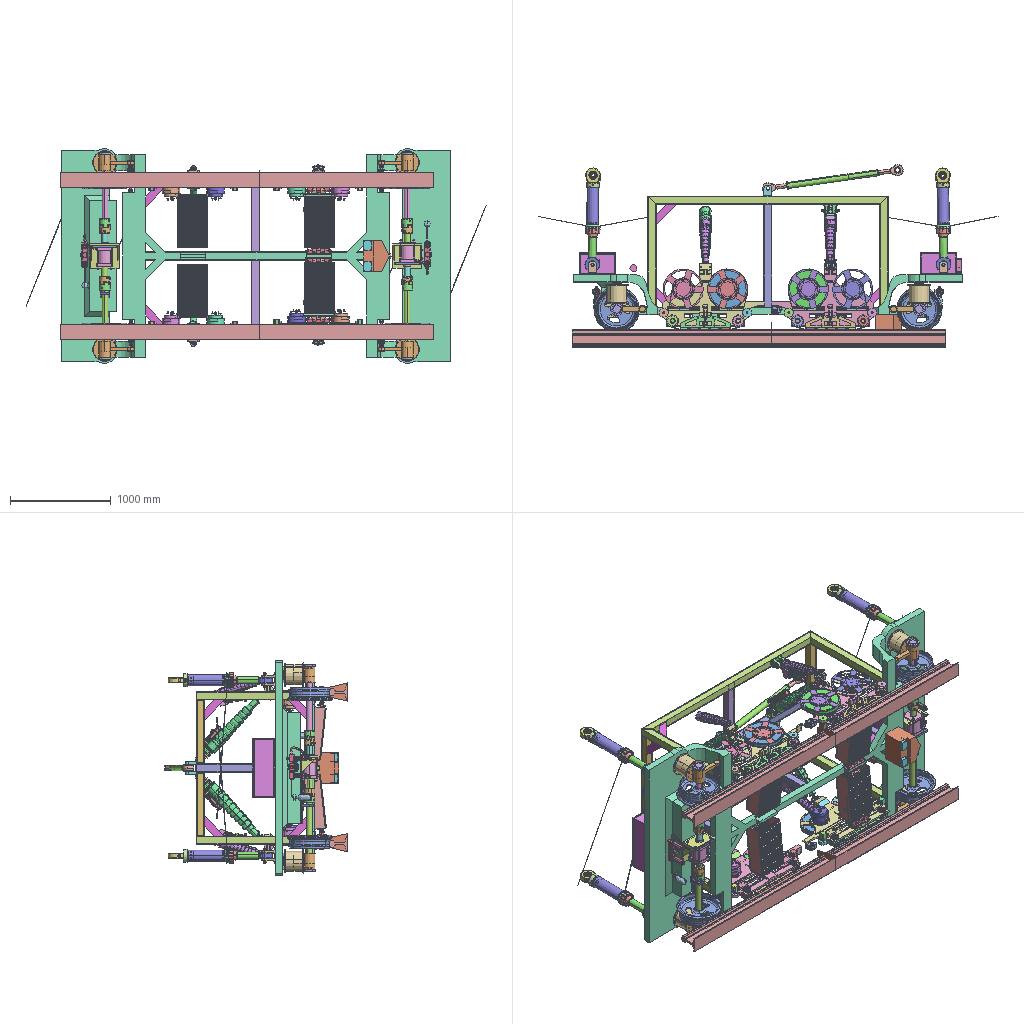Assembly | STEP file | 122 different items | 810 placed | box 4562 x 1815 x 2130 mm
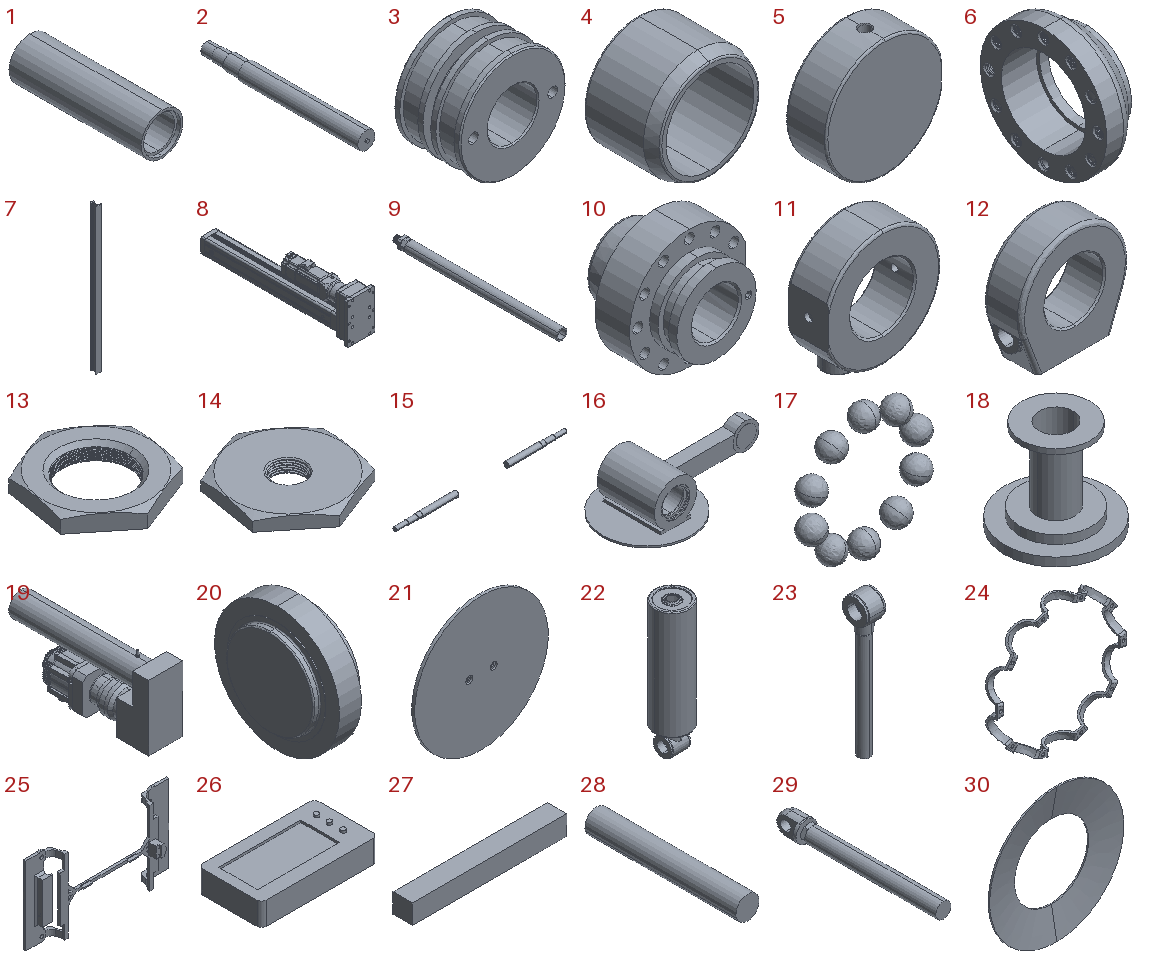Parts list (item | name | quantity | parent item | size | volume):
1 | 1. Barrel | x4 | in Hydraulic cylinder | 114.3 x 362.5 x 114.3 mm | 1450450 mm3
2 | 2. Piston Rod | x4 | in Hydraulic cylinder | 71.582 x 670.101 x 71.582 mm | 2394238 mm3
3 | 3. Piston | x4 | in Hydraulic cylinder | 88.35 x 55 x 88.35 mm | 216858 mm3
4 | 4. Piston Cap | x4 | in Hydraulic cylinder | 60 x 40 x 60 mm | 35974 mm3
5 | 5. End Cap | x4 | in Hydraulic cylinder | - | -
6 | 6. Barrel Cap | x4 | in Hydraulic cylinder | - | -
7 | 60 rail | x2 | - | 150 x 176.167 x 3700 mm | 28206021 mm3
8 | 60-400mm cylinder body | x2 | in 60-400mm branch 12 | - | -
9 | 60-400mm push rod | x2 | in 60-400mm branch 12 | 35 x 555 x 35 mm | 228632 mm3
10 | 7. Front Cap | x4 | in Hydraulic cylinder | - | -
11 | 8. Front Clevis | x4 | in Hydraulic cylinder | - | -
12 | 9. Rear Clevis | x4 | in Hydraulic cylinder | 146 x 50.8 x 148 mm | 646716 mm3
13 | Adjusting nut 1 | x4 | in Axle box spring | 86.085 x 91.305 x 12 mm | 42133 mm3
14 | Adjusting nut 2 | x4 | in VSVDMRD | 53.803 x 57.066 x 6 mm | 11857 mm3
15 | Axle | x2 | - | 2025 x 64 x 64 mm | 3440421 mm3
16 | Axle box 1 | x4 | - | 410 x 240 x 120.8 mm | 1300329 mm3
17 | Ball | x16 | in Ball Bearing | 70.063 x 13 x 73 mm | 11503 mm3
18 | Base | x4 | in VSVDMRD | 60 x 60 x 53 mm | 24076 mm3
19 | Base body | x2 | in Multi-stage cylinder assembly | 90 x 360 x 196.75 mm | 2809262 mm3
20 | Bearing end cap 1 | x4 | - | 39.936 x 120.436 x 120.436 mm | 192561 mm3
21 | Bottom cover | x4 | in Housing assembly | 230 x 5 x 230 mm | 206946 mm3
22 | C40-55H | x4 | in 22 | - | -
23 | C40-55H-1 | x4 | in 22 | - | -
24 | Case | x32 | in Ball Bearing | 63.56 x 7.5 x 63.56 mm | 756.109 mm3
25 | Chassis | x1 | - | 3860 x 630 x 2130 mm | 286011654 mm3
26 | Controller | x1 | - | 254.791 x 138.794 x 55 mm | 1688527 mm3
27 | Crossbeam | x3 | - | 635 x 80 x 80 mm | 1850000 mm3
28 | Cylinder 1 | x2 | in Multi-stage cylinder assembly | 46 x 300 x 46 mm | 498571 mm3
29 | Cylinder 2 | x2 | in Multi-stage cylinder assembly | 48 x 372 x 48.4 mm | 366109 mm3
30 | Disc spring | x48 | in Disc spring stack | 90 x 4.485 x 90 mm | 4464 mm3
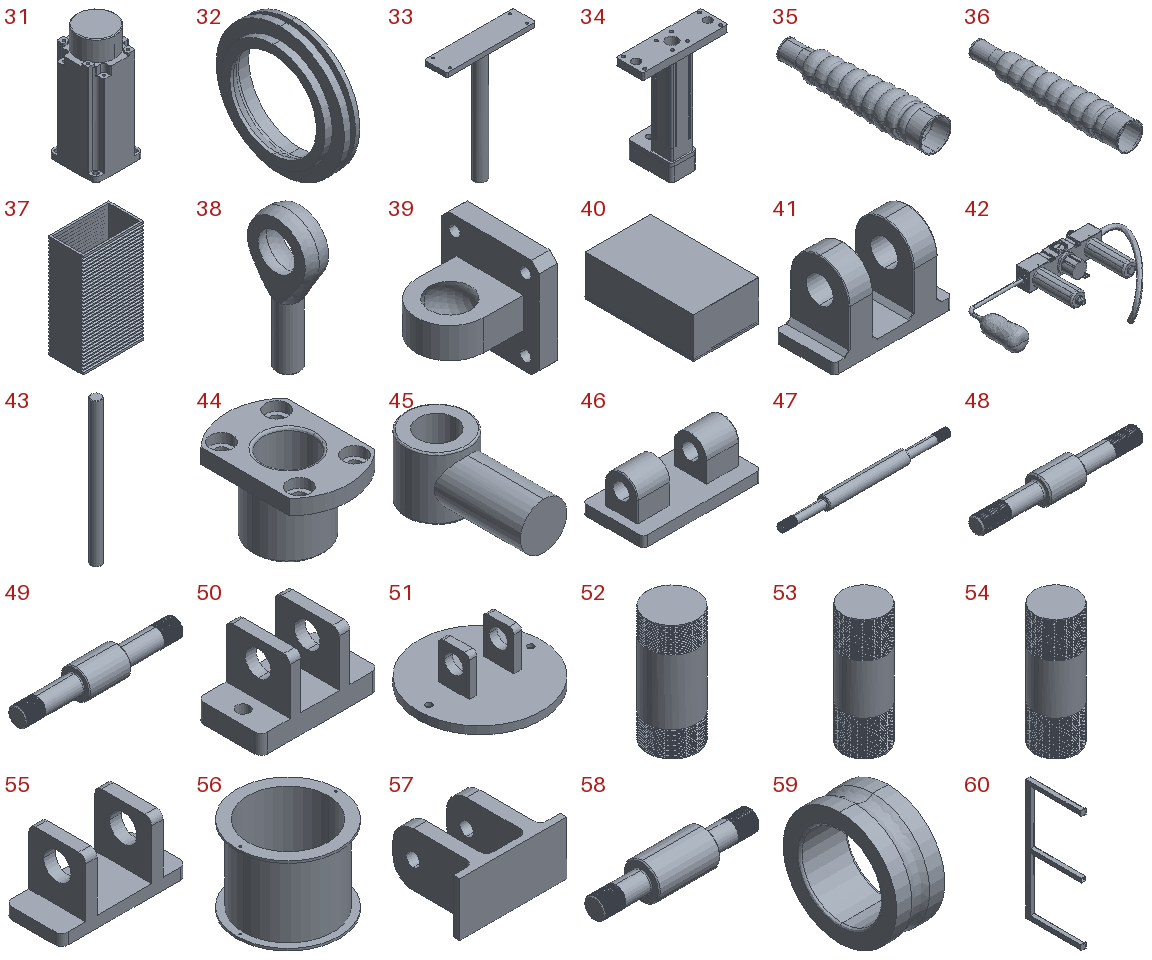31 | Drive motor | x2 | in Electric cylinder with guide post | 60 x 60 x 146.5 mm | 432413 mm3
32 | Dust ring 1 | x2 | - | 15.692 x 75.322 x 75.322 mm | 18737 mm3
33 | Electric cylinder assembly 1 | x2 | in Electric cylinder with guide post | 295 x 75 x 394 mm | 805333 mm3
34 | Electric cylinder assembly 2 | x2 | in Electric cylinder with guide post | 295 x 157.01 x 389 mm | 2717250 mm3
35 | Electric cylinder dust boot, cylinder A | x4 | - | 98.284 x 439.582 x 98.284 mm | 200790 mm3
36 | Electric cylinder dust boot, cylinder B | x4 | - | 122.855 x 671.584 x 122.855 mm | 479397 mm3
37 | Electric cylinder dust boot, cylinder C | x4 | - | 300 x 172 x 510 mm | 3753035 mm3
38 | Electric cylinder end | x2 | in 60-400mm branch 12 | 20 x 53.333 x 116.667 mm | 46086 mm3
39 | Electric cylinder rear end | x2 | in 60-400mm branch 12 | 102.201 x 110.238 x 110 mm | 342239 mm3
40 | Electrical box | x2 | - | - | 11408010 mm3
41 | Frame R-pair hinge lug | x4 | in 打磨单元与电动缸-3支链-铰接点加宽, 打磨单元与电动缸Mirror-3支链-铰接点加宽 | 140 x 70 x 98 mm | 392765 mm3
42 | GC300-400 FRL air unit [GC400-15]_GC400-15 | x2 | in CS2 series standard pneumatic cylinder [CDS2F140-100]_CDS2F140-100 | 534.272 x 247.073 x 161.659 mm | 1621507 mm3
43 | Guide post | x4 | in Electric cylinder with guide post | 20 x 20 x 280 mm | 87904 mm3
44 | Guide post flange | x4 | in Electric cylinder with guide post | 34 x 49 x 30 mm | 13227 mm3
45 | Hinge | x4 | in VSVDMRD | 20 x 44.5 x 20 mm | 8479 mm3
46 | Hinge lug widened | x4 | in Electric cylinder with guide post | 145 x 75 x 58 mm | 246181 mm3
47 | Hinge pin stepped shaft | x4 | in Hinge assembly M20 spacing 20 | 260 x 20 x 20 mm | 54217 mm3
48 | Hinge pin stepped shaft 1 | x4 | in Unit hinge short shaft | 120 x 20 x 20 mm | 18916 mm3
49 | Hinge pin stepped shaft 2 | x4 | in Frame hinge short shaft | 172 x 32 x 32 mm | 76081 mm3
50 | Hinge seat | x4 | in Axle box spring | 55 x 30 x 34 mm | 20602 mm3
51 | Hinge seat 1 | x4 | in Axle box spring | 80 x 80 x 30 mm | 28682 mm3
52 | Hinge seat cylinder | x4 | in Axle box spring | 12 x 12 x 28 mm | 3114 mm3
53 | Hinge seat cylinder 1 | x4 | in Axle box spring | 12 x 12 x 34 mm | 3769 mm3
54 | Hinge seat cylinder 3 | x8 | in VSVDMRD | 12 x 12 x 34 mm | 3769 mm3
55 | Hinge top seat 3 | x8 | in VSVDMRD | 55 x 25 x 30 mm | 11917 mm3
56 | Housing | x4 | in Housing assembly | 230 x 230 x 175 mm | 1145645 mm3
57 | Hydraulic cylinder base | x4 | - | 160 x 130 x 80 mm | 490850 mm3
58 | Hydraulic cylinder hinge pin stepped shaft | x4 | - | 152 x 35 x 35 mm | 86130 mm3
59 | Inner Ring | x16 | in Ball Bearing | 21 x 49.56 x 49.56 mm | 19228 mm3
60 | Inner frame 1 | x1 | - | 100 x 1100 x 2400 mm | 8328429 mm3
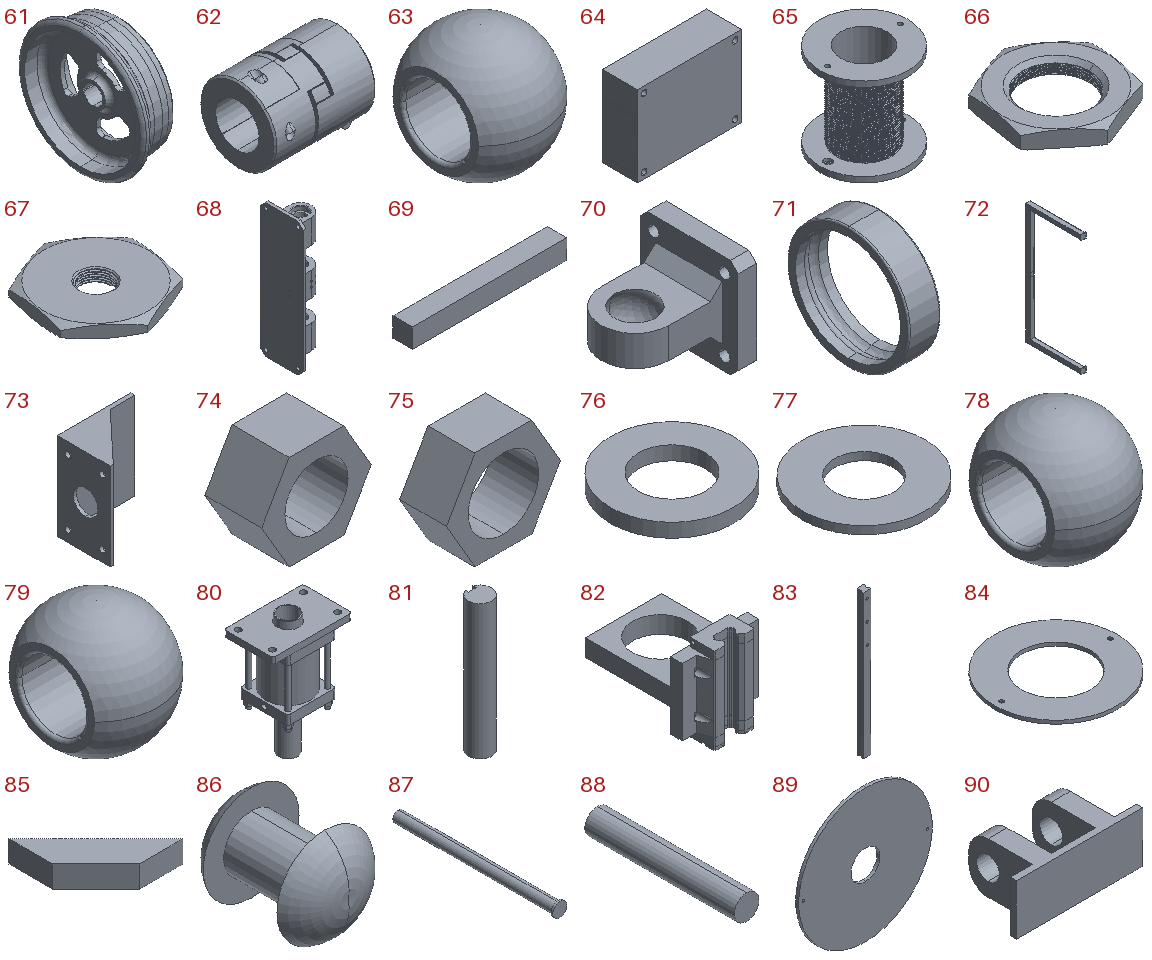61 | LM wheel | x4 | - | 135 x 449.742 x 449.742 mm | 4161570 mm3
62 | LYCA jaw coupling [LYCA-105140]_LYCA-105140 | x4 | in CS2 series standard pneumatic cylinder [CDS2F140-100]_CDS2F140-100 | 140 x 108.875 x 107.681 mm | 781609 mm3
63 | Large rod end bearing | x2 | in 60-400mm branch 12 | 42.667 x 59.28 x 59.28 mm | 62997 mm3
64 | Laser ranging sensor 1200mm | x2 | - | 92 x 31 x 71 mm | 199839 mm3
65 | Load-bearing column 1 | x4 | in Axle box spring | 80 x 80 x 80 mm | 74344 mm3
66 | Lock nut | x4 | in Axle box spring | 86.085 x 91.305 x 12 mm | 41343 mm3
67 | Lock nut 2 | x4 | in VSVDMRD | 53.803 x 57.066 x 6 mm | 11722 mm3
68 | Lower hinge plate thickness 20 widened | x4 | in 打磨单元与电动缸-3支链-铰接点加宽, 打磨单元与电动缸Mirror-3支链-铰接点加宽 | 55 x 80 x 248 mm | 298124 mm3
69 | Middle crossbeam | x2 | - | 635 x 80 x 80 mm | 1850000 mm3
70 | Multi-stage electric cylinder rear end | x2 | in Multi-stage cylinder assembly | 90.745 x 85.184 x 85 mm | 182065 mm3
71 | Outer Ring | x16 | in Ball Bearing | 21 x 80 x 80 mm | 23803 mm3
72 | Outer frame 1 | x2 | - | 100 x 1100 x 2400 mm | 6796800 mm3
73 | Part 2 | x2 | - | 240 x 172.72 x 285 mm | 1617851 mm3
74 | Pin shaft nut M12 | x16 | in Hinge assembly M20 spacing 20, Unit hinge short shaft | 20.785 x 10.8 x 18 mm | 1809 mm3
75 | Pin shaft nut M20 | x8 | in Frame hinge short shaft | 32.332 x 13.3 x 28 mm | 4852 mm3
76 | Pin washer nut at M12 | x8 | in Unit hinge short shaft | 24 x 24 x 2.7 mm | 863.074 mm3
77 | Pin washer nut at M20 | x8 | in Frame hinge short shaft | 42 x 42 x 2.7 mm | 2892 mm3
78 | Rod end bearing | x2 | in 60-400mm branch 12 | 26.667 x 37.05 x 37.05 mm | 15380 mm3
79 | Rod end bearing 1 | x2 | in Traction tie rod | 56 x 77.805 x 77.805 mm | 142436 mm3
80 | - | x2 | in CS2 series standard pneumatic cylinder [CDS2F140-100]_CDS2F140-100 | 255 x 160 x 391 mm | 4492396 mm3
81 | - | x2 | in CS2 series standard pneumatic cylinder [CDS2F140-100]_CDS2F140-100 | 60 x 60 x 350 mm | 980167 mm3
82 | - | x2 | in HGW-CC, HGW-HC ball linear guide [HGW25HCE1R160EZ0CI+E2╱RC] | 90 x 130.4 x 101.35 mm | 273485 mm3
83 | - | x2 | in HGW-CC, HGW-HC ball linear guide [HGW25HCE1R160EZ0CI+E2╱RC] | 23 x 22 x 429 mm | 189571 mm3
84 | Spacer block | x4 | in Axle box spring | 180 x 180 x 5 mm | 87215 mm3
85 | Support rib 1 | x10 | - | 200 x 200 x 50 mm | 750000 mm3
86 | Szegecs | x160 | in Ball Bearing | 2.6 x 3.322 x 2.6 mm | 7.735 mm3
87 | Tie rod | x1 | in Traction tie rod | 80 x 910 x 80 mm | 827810 mm3
88 | Tie rod 2 | x1 | in Traction tie rod | 50 x 300 x 50 mm | 589049 mm3
89 | Top cover | x4 | in Housing assembly | 230 x 5 x 230 mm | 197795 mm3
90 | Traction rod base | x1 | in Traction tie rod | 200 x 110 x 80 mm | 555750 mm3
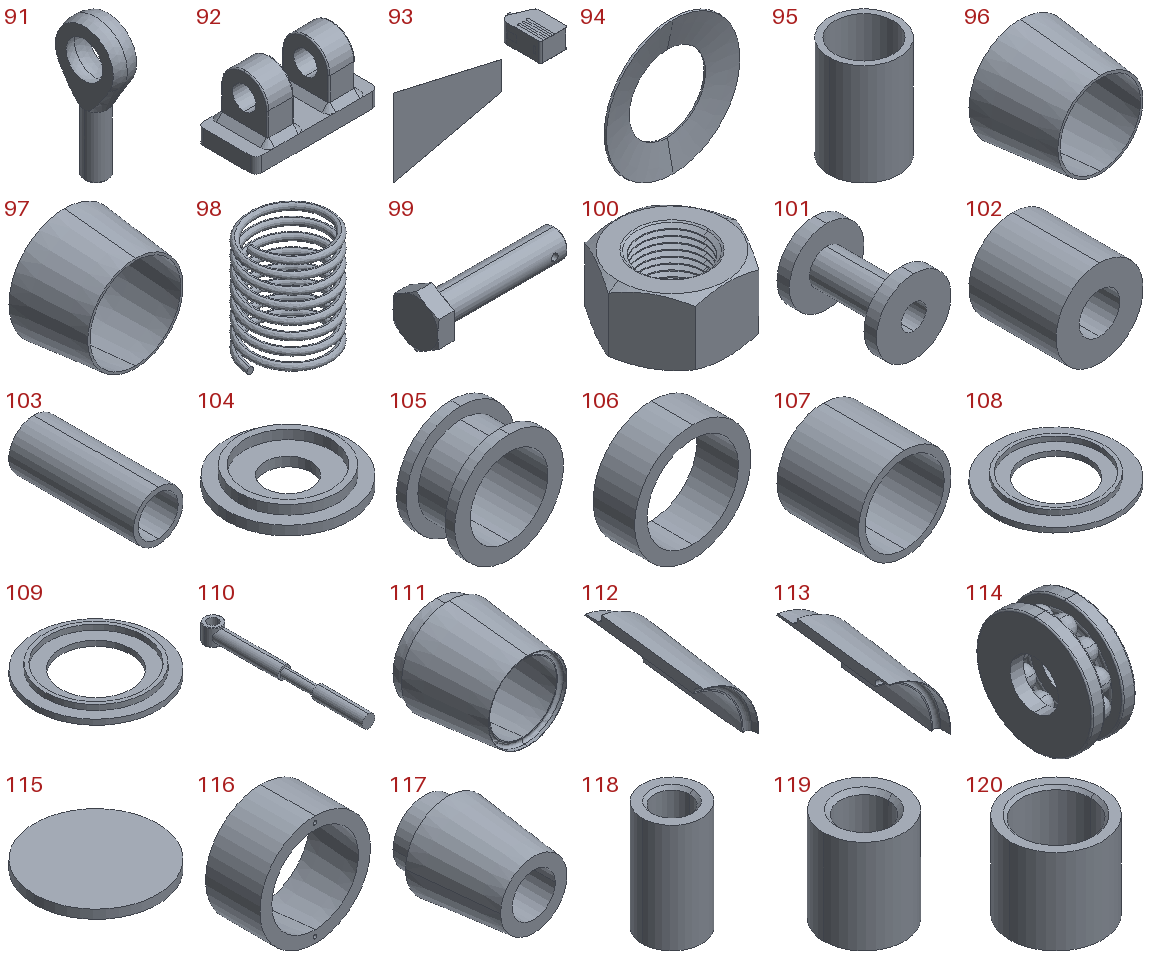91 | Traction rod end | x2 | in Traction tie rod | 42 x 112 x 245 mm | 426798 mm3
92 | Unit R-pair hinge lug | x4 | in 打磨单元与电动缸-3支链-铰接点加宽, 打磨单元与电动缸Mirror-3支链-铰接点加宽 | 105 x 50 x 58 mm | 130356 mm3
93 | ZLDS202_250 | x2 | in 打磨单元与电动缸-3支链-铰接点加宽, 打磨单元与电动缸Mirror-3支链-铰接点加宽 | 403 x 111.961 x 180 mm | 243934 mm3
94 | disc spring2 | x40 | in disc spring group2 | 70.392 x 3.981 x 70.392 mm | 2653 mm3
95 | end shield | x1 | in VSVDMRD | 24 x 24 x 35 mm | 6409 mm3
96 | getao1 | x4 | in rubber | 126.7 x 99.651 x 126.7 mm | 106341 mm3
97 | getao2 | x4 | in rubber | 146 x 94.195 x 146 mm | 118161 mm3
98 | helical spring | x4 | in VSVDMRD | 49.976 x 49.976 x 68 mm | 14534 mm3
99 | hex bolts split pin hole-fine pitch-ab gb_PreviewCfg | x44 | in Hydraulic cylinder | 40.3 x 13 x 15.011 mm | 2490 mm3
100 | hex nuts, style 1-grades ab gb_GB_FASTENER_NUT_SNAB1  B M20-S | x7 | - | 34.641 x 30 x 18 mm | 9181 mm3
101 | inner coil1 | x4 | in VSVDMRD | 30 x 40 x 30 mm | 8545 mm3
102 | inner coil2 | x4 | in VSVDMRD | 30 x 30 x 30 mm | 16588 mm3
103 | inner cylinder block | x4 | in VSVDMRD | 40 x 100 x 40 mm | 45239 mm3
104 | inner seal | x8 | in VSVDMRD | 40 x 40 x 6 mm | 3805 mm3
105 | outer coil1 | x4 | in VSVDMRD | 56 x 30 x 56 mm | 17342 mm3
106 | outer coil2 | x4 | in VSVDMRD | 56 x 20 x 56 mm | 18850 mm3
107 | outer cylinder block | x4 | in VSVDMRD | 68 x 60 x 68 mm | 59376 mm3
108 | outer seal | x4 | in VSVDMRD | 76 x 76 x 6 mm | 10895 mm3
109 | outer seal2 | x4 | in VSVDMRD | 70 x 70 x 6 mm | 8831 mm3
110 | piston rod | x4 | in VSVDMRD | 20 x 194.5 x 20 mm | 31059 mm3
111 | rubber1 | x4 | in rubber | 120.71 x 115.719 x 120.71 mm | 254133 mm3
112 | rubber2 | x8 | in rubber | 60.803 x 107.596 x 68.922 mm | 62752 mm3
113 | rubber3 | x8 | in rubber | 68.197 x 105.496 x 77.952 mm | 66050 mm3
114 | thrust ball bearings gb_PreviewCfg | x8 | in Hinge assembly M20 spacing 20 | 9 x 24 x 24 mm | 2455 mm3
115 | top cover | x1 | in VSVDMRD | 70 x 70 x 5 mm | 19242 mm3
116 | waitao | x4 | in rubber | 178.3 x 87.518 x 178.3 mm | 654591 mm3
117 | zhouxin | x4 | in rubber | 108 x 140 x 108 mm | 645082 mm3
118 | 塑料轴套内10外20长20 | x8 | in Hinge assembly M20 spacing 20 | 20 x 20 x 36.7 mm | 7339 mm3
119 | 塑料轴套内10外20长20 Copy | x8 | in Unit hinge short shaft | 20 x 20 x 23.5 mm | 4685 mm3
120 | 塑料轴套内10外20长20 Copy 2 | x8 | in Frame hinge short shaft | 32 x 32 x 29.5 mm | 10302 mm3
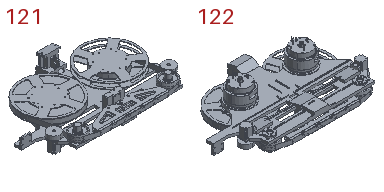121 | 打磨单元方案20250311-1-第二版 | x2 | in 打磨单元与电动缸-3支链-铰接点加宽 | - | 21551656 mm3
122 | 打磨单元方案20250311-1-第二版_MirrorDefault | x2 | in 打磨单元与电动缸Mirror-3支链-铰接点加宽 | - | 21550572 mm3